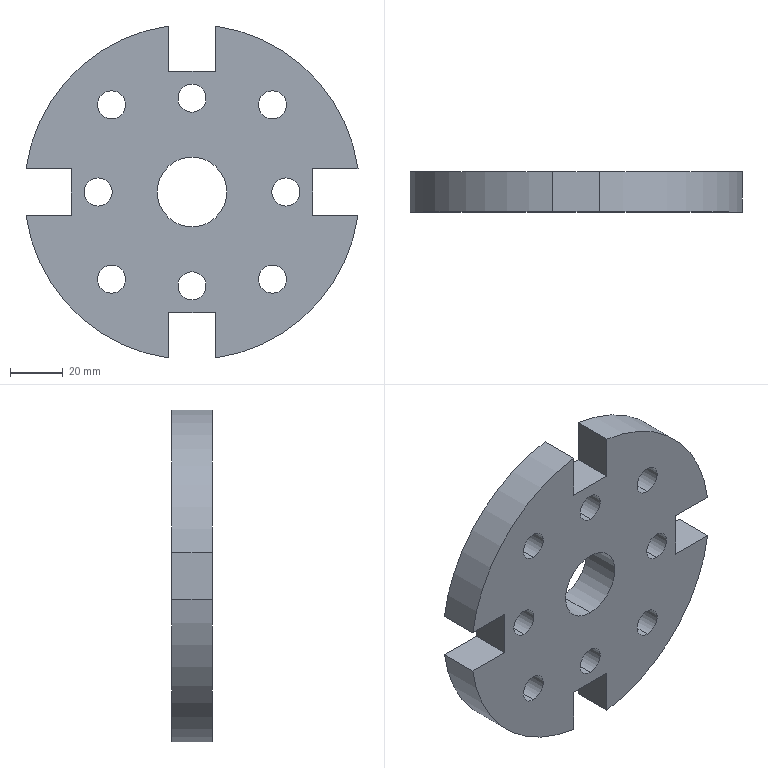Part | SolidWorks | features ICE 2, CirPattern 1, Extrusion 1, Scale 1 | 1 solid | 36 faces | box 125.749 x 15.24 x 125.749 mm | volume 154760 mm3 | cylinder 22 | plane 14 | commonest cylinder face diameters 10.668 x16 127 x4 26.416 x2
STEP:
#1=CARTESIAN_POINT('',(0.,-15.24,30.226));
#2=VERTEX_POINT('',#1);
#3=CARTESIAN_POINT('',(0.,-15.24,40.894));
#4=VERTEX_POINT('',#3);
#5=CARTESIAN_POINT('',(0.,-15.24,35.56));
#6=DIRECTION('',(0.,1.,0.));
#7=DIRECTION('',(0.,0.,1.));
#8=AXIS2_PLACEMENT_3D('',#5,#6,#7);
#9=CIRCLE('',#8,5.334);
#10=EDGE_CURVE('',#2,#4,#9,.T.);
#11=ORIENTED_EDGE('',*,*,#10,.F.);
#12=CARTESIAN_POINT('',(0.,0.,30.226));
#13=VERTEX_POINT('',#12);
#14=CARTESIAN_POINT('',(0.,-15.24,30.226));
#15=DIRECTION('',(0.,1.,0.));
#16=VECTOR('',#15,1000.);
#17=LINE('',#14,#16);
#18=EDGE_CURVE('',#2,#13,#17,.T.);
#19=ORIENTED_EDGE('',*,*,#18,.T.);
#20=CARTESIAN_POINT('',(0.,0.,40.894));
#21=VERTEX_POINT('',#20);
#22=CARTESIAN_POINT('',(0.,0.,35.56));
#23=DIRECTION('',(0.,1.,0.));
#24=DIRECTION('',(0.,0.,1.));
#25=AXIS2_PLACEMENT_3D('',#22,#23,#24);
#26=CIRCLE('',#25,5.334);
#27=EDGE_CURVE('',#13,#21,#26,.T.);
#28=ORIENTED_EDGE('',*,*,#27,.T.);
#29=CARTESIAN_POINT('',(0.,-15.24,40.894));
#30=DIRECTION('',(0.,1.,0.));
#31=VECTOR('',#30,1000.);
#32=LINE('',#29,#31);
#33=EDGE_CURVE('',#4,#21,#32,.T.);
#34=ORIENTED_EDGE('',*,*,#33,.F.);
#35=EDGE_LOOP('',(#11,#19,#28,#34));
#36=FACE_OUTER_BOUND('',#35,.T.);
#37=CARTESIAN_POINT('',(0.,-15.24,35.56));
#38=DIRECTION('',(0.,1.,0.));
#39=DIRECTION('',(0.,0.,1.));
#40=AXIS2_PLACEMENT_3D('',#37,#38,#39);
#41=CYLINDRICAL_SURFACE('',#40,5.334);
#42=ADVANCED_FACE('',(#36),#41,.F.);
#43=CARTESIAN_POINT('',(35.56,-15.24,-5.334));
#44=VERTEX_POINT('',#43);
#45=CARTESIAN_POINT('',(35.56,-15.24,5.334));
#46=VERTEX_POINT('',#45);
#47=CARTESIAN_POINT('',(35.56,-15.24,0.));
#48=DIRECTION('',(0.,1.,0.));
#49=DIRECTION('',(0.,0.,1.));
#50=AXIS2_PLACEMENT_3D('',#47,#48,#49);
#51=CIRCLE('',#50,5.334);
#52=EDGE_CURVE('',#44,#46,#51,.T.);
#53=ORIENTED_EDGE('',*,*,#52,.F.);
#54=CARTESIAN_POINT('',(35.56,0.,-5.334));
#55=VERTEX_POINT('',#54);
#56=CARTESIAN_POINT('',(35.56,-15.24,-5.334));
#57=DIRECTION('',(0.,1.,0.));
#58=VECTOR('',#57,1000.);
#59=LINE('',#56,#58);
#60=EDGE_CURVE('',#44,#55,#59,.T.);
#61=ORIENTED_EDGE('',*,*,#60,.T.);
#62=CARTESIAN_POINT('',(35.56,0.,5.334));
#63=VERTEX_POINT('',#62);
#64=CARTESIAN_POINT('',(35.56,0.,0.));
#65=DIRECTION('',(0.,1.,0.));
#66=DIRECTION('',(0.,0.,1.));
#67=AXIS2_PLACEMENT_3D('',#64,#65,#66);
#68=CIRCLE('',#67,5.334);
#69=EDGE_CURVE('',#55,#63,#68,.T.);
#70=ORIENTED_EDGE('',*,*,#69,.T.);
#71=CARTESIAN_POINT('',(35.56,-15.24,5.334));
#72=DIRECTION('',(0.,1.,0.));
#73=VECTOR('',#72,1000.);
#74=LINE('',#71,#73);
#75=EDGE_CURVE('',#46,#63,#74,.T.);
#76=ORIENTED_EDGE('',*,*,#75,.F.);
#77=EDGE_LOOP('',(#53,#61,#70,#76));
#78=FACE_OUTER_BOUND('',#77,.T.);
#79=CARTESIAN_POINT('',(35.56,-15.24,0.));
#80=DIRECTION('',(0.,1.,0.));
#81=DIRECTION('',(0.,0.,1.));
#82=AXIS2_PLACEMENT_3D('',#79,#80,#81);
#83=CYLINDRICAL_SURFACE('',#82,5.334);
#84=ADVANCED_FACE('',(#78),#83,.F.);
#85=CARTESIAN_POINT('',(0.,-15.24,-40.894));
#86=VERTEX_POINT('',#85);
#87=CARTESIAN_POINT('',(0.,-15.24,-30.226));
#88=VERTEX_POINT('',#87);
#89=CARTESIAN_POINT('',(0.,-15.24,-35.56));
#90=DIRECTION('',(0.,1.,0.));
#91=DIRECTION('',(0.,0.,1.));
#92=AXIS2_PLACEMENT_3D('',#89,#90,#91);
#93=CIRCLE('',#92,5.334);
#94=EDGE_CURVE('',#86,#88,#93,.T.);
#95=ORIENTED_EDGE('',*,*,#94,.F.);
#96=CARTESIAN_POINT('',(0.,0.,-40.894));
#97=VERTEX_POINT('',#96);
#98=CARTESIAN_POINT('',(0.,-15.24,-40.894));
#99=DIRECTION('',(0.,1.,0.));
#100=VECTOR('',#99,1000.);
#101=LINE('',#98,#100);
#102=EDGE_CURVE('',#86,#97,#101,.T.);
#103=ORIENTED_EDGE('',*,*,#102,.T.);
#104=CARTESIAN_POINT('',(0.,0.,-30.226));
#105=VERTEX_POINT('',#104);
#106=CARTESIAN_POINT('',(0.,0.,-35.56));
#107=DIRECTION('',(0.,1.,0.));
#108=DIRECTION('',(0.,0.,1.));
#109=AXIS2_PLACEMENT_3D('',#106,#107,#108);
#110=CIRCLE('',#109,5.334);
#111=EDGE_CURVE('',#97,#105,#110,.T.);
#112=ORIENTED_EDGE('',*,*,#111,.T.);
#113=CARTESIAN_POINT('',(0.,-15.24,-30.226));
#114=DIRECTION('',(0.,1.,0.));
#115=VECTOR('',#114,1000.);
#116=LINE('',#113,#115);
#117=EDGE_CURVE('',#88,#105,#116,.T.);
#118=ORIENTED_EDGE('',*,*,#117,.F.);
#119=EDGE_LOOP('',(#95,#103,#112,#118));
#120=FACE_OUTER_BOUND('',#119,.T.);
#121=CARTESIAN_POINT('',(0.,-15.24,-35.56));
#122=DIRECTION('',(0.,1.,0.));
#123=DIRECTION('',(0.,0.,1.));
#124=AXIS2_PLACEMENT_3D('',#121,#122,#123);
#125=CYLINDRICAL_SURFACE('',#124,5.334);
#126=ADVANCED_FACE('',(#120),#125,.F.);
#127=CARTESIAN_POINT('',(-35.56,-15.24,-5.334));
#128=VERTEX_POINT('',#127);
#129=CARTESIAN_POINT('',(-35.56,-15.24,5.334));
#130=VERTEX_POINT('',#129);
#131=CARTESIAN_POINT('',(-35.56,-15.24,0.));
#132=DIRECTION('',(0.,1.,0.));
#133=DIRECTION('',(0.,0.,1.));
#134=AXIS2_PLACEMENT_3D('',#131,#132,#133);
#135=CIRCLE('',#134,5.334);
#136=EDGE_CURVE('',#128,#130,#135,.T.);
#137=ORIENTED_EDGE('',*,*,#136,.F.);
#138=CARTESIAN_POINT('',(-35.56,0.,-5.334));
#139=VERTEX_POINT('',#138);
#140=CARTESIAN_POINT('',(-35.56,-15.24,-5.334));
#141=DIRECTION('',(0.,1.,0.));
#142=VECTOR('',#141,1000.);
#143=LINE('',#140,#142);
#144=EDGE_CURVE('',#128,#139,#143,.T.);
#145=ORIENTED_EDGE('',*,*,#144,.T.);
#146=CARTESIAN_POINT('',(-35.56,0.,5.334));
#147=VERTEX_POINT('',#146);
#148=CARTESIAN_POINT('',(-35.56,0.,0.));
#149=DIRECTION('',(0.,1.,0.));
#150=DIRECTION('',(0.,0.,1.));
#151=AXIS2_PLACEMENT_3D('',#148,#149,#150);
#152=CIRCLE('',#151,5.334);
#153=EDGE_CURVE('',#139,#147,#152,.T.);
#154=ORIENTED_EDGE('',*,*,#153,.T.);
#155=CARTESIAN_POINT('',(-35.56,-15.24,5.334));
#156=DIRECTION('',(0.,1.,0.));
#157=VECTOR('',#156,1000.);
#158=LINE('',#155,#157);
#159=EDGE_CURVE('',#130,#147,#158,.T.);
#160=ORIENTED_EDGE('',*,*,#159,.F.);
#161=EDGE_LOOP('',(#137,#145,#154,#160));
#162=FACE_OUTER_BOUND('',#161,.T.);
#163=CARTESIAN_POINT('',(-35.56,-15.24,0.));
#164=DIRECTION('',(0.,1.,0.));
#165=DIRECTION('',(0.,0.,1.));
#166=AXIS2_PLACEMENT_3D('',#163,#164,#165);
#167=CYLINDRICAL_SURFACE('',#166,5.334);
#168=ADVANCED_FACE('',(#162),#167,.F.);
#169=CARTESIAN_POINT('',(0.,-15.24,-13.208));
#170=VERTEX_POINT('',#169);
#171=CARTESIAN_POINT('',(0.,-15.24,13.208));
#172=VERTEX_POINT('',#171);
#173=CARTESIAN_POINT('',(0.,-15.24,0.));
#174=DIRECTION('',(0.,1.,0.));
#175=DIRECTION('',(0.,0.,1.));
#176=AXIS2_PLACEMENT_3D('',#173,#174,#175);
#177=CIRCLE('',#176,13.208);
#178=EDGE_CURVE('',#170,#172,#177,.T.);
#179=ORIENTED_EDGE('',*,*,#178,.F.);
#180=CARTESIAN_POINT('',(0.,0.,-13.208));
#181=VERTEX_POINT('',#180);
#182=CARTESIAN_POINT('',(0.,-15.24,-13.208));
#183=DIRECTION('',(0.,1.,0.));
#184=VECTOR('',#183,1000.);
#185=LINE('',#182,#184);
#186=EDGE_CURVE('',#170,#181,#185,.T.);
#187=ORIENTED_EDGE('',*,*,#186,.T.);
#188=CARTESIAN_POINT('',(0.,0.,13.208));
#189=VERTEX_POINT('',#188);
#190=CARTESIAN_POINT('',(0.,0.,0.));
#191=DIRECTION('',(0.,1.,0.));
#192=DIRECTION('',(0.,0.,1.));
#193=AXIS2_PLACEMENT_3D('',#190,#191,#192);
#194=CIRCLE('',#193,13.208);
#195=EDGE_CURVE('',#181,#189,#194,.T.);
#196=ORIENTED_EDGE('',*,*,#195,.T.);
#197=CARTESIAN_POINT('',(0.,-15.24,13.208));
#198=DIRECTION('',(0.,1.,0.));
#199=VECTOR('',#198,1000.);
#200=LINE('',#197,#199);
#201=EDGE_CURVE('',#172,#189,#200,.T.);
#202=ORIENTED_EDGE('',*,*,#201,.F.);
#203=EDGE_LOOP('',(#179,#187,#196,#202));
#204=FACE_OUTER_BOUND('',#203,.T.);
#205=CARTESIAN_POINT('',(0.,-15.24,0.));
#206=DIRECTION('',(0.,1.,0.));
#207=DIRECTION('',(0.,0.,1.));
#208=AXIS2_PLACEMENT_3D('',#205,#206,#207);
#209=CYLINDRICAL_SURFACE('',#208,13.208);
#210=ADVANCED_FACE('',(#204),#209,.F.);
#211=CARTESIAN_POINT('',(-30.48,-15.24,27.686));
#212=VERTEX_POINT('',#211);
#213=CARTESIAN_POINT('',(-30.48,-15.24,38.354));
#214=VERTEX_POINT('',#213);
#215=CARTESIAN_POINT('',(-30.48,-15.24,33.02));
#216=DIRECTION('',(0.,1.,0.));
#217=DIRECTION('',(0.,0.,1.));
#218=AXIS2_PLACEMENT_3D('',#215,#216,#217);
#219=CIRCLE('',#218,5.334);
#220=EDGE_CURVE('',#212,#214,#219,.T.);
#221=ORIENTED_EDGE('',*,*,#220,.F.);
#222=CARTESIAN_POINT('',(-30.48,0.,27.686));
#223=VERTEX_POINT('',#222);
#224=CARTESIAN_POINT('',(-30.48,-15.24,27.686));
#225=DIRECTION('',(0.,1.,0.));
#226=VECTOR('',#225,1000.);
#227=LINE('',#224,#226);
#228=EDGE_CURVE('',#212,#223,#227,.T.);
#229=ORIENTED_EDGE('',*,*,#228,.T.);
#230=CARTESIAN_POINT('',(-30.48,0.,38.354));
#231=VERTEX_POINT('',#230);
#232=CARTESIAN_POINT('',(-30.48,0.,33.02));
#233=DIRECTION('',(0.,1.,0.));
#234=DIRECTION('',(0.,0.,1.));
#235=AXIS2_PLACEMENT_3D('',#232,#233,#234);
#236=CIRCLE('',#235,5.334);
#237=EDGE_CURVE('',#223,#231,#236,.T.);
#238=ORIENTED_EDGE('',*,*,#237,.T.);
#239=CARTESIAN_POINT('',(-30.48,-15.24,38.354));
#240=DIRECTION('',(0.,1.,0.));
#241=VECTOR('',#240,1000.);
#242=LINE('',#239,#241);
#243=EDGE_CURVE('',#214,#231,#242,.T.);
#244=ORIENTED_EDGE('',*,*,#243,.F.);
#245=EDGE_LOOP('',(#221,#229,#238,#244));
#246=FACE_OUTER_BOUND('',#245,.T.);
#247=CARTESIAN_POINT('',(-30.48,-15.24,33.02));
#248=DIRECTION('',(0.,1.,0.));
#249=DIRECTION('',(0.,0.,1.));
#250=AXIS2_PLACEMENT_3D('',#247,#248,#249);
#251=CYLINDRICAL_SURFACE('',#250,5.334);
#252=ADVANCED_FACE('',(#246),#251,.F.);
#253=CARTESIAN_POINT('',(30.48,-15.24,27.686));
#254=VERTEX_POINT('',#253);
#255=CARTESIAN_POINT('',(30.48,-15.24,38.354));
#256=VERTEX_POINT('',#255);
#257=CARTESIAN_POINT('',(30.48,-15.24,33.02));
#258=DIRECTION('',(0.,1.,0.));
#259=DIRECTION('',(0.,0.,1.));
#260=AXIS2_PLACEMENT_3D('',#257,#258,#259);
#261=CIRCLE('',#260,5.334);
#262=EDGE_CURVE('',#254,#256,#261,.T.);
#263=ORIENTED_EDGE('',*,*,#262,.F.);
#264=CARTESIAN_POINT('',(30.48,0.,27.686));
#265=VERTEX_POINT('',#264);
#266=CARTESIAN_POINT('',(30.48,-15.24,27.686));
#267=DIRECTION('',(0.,1.,0.));
#268=VECTOR('',#267,1000.);
#269=LINE('',#266,#268);
#270=EDGE_CURVE('',#254,#265,#269,.T.);
#271=ORIENTED_EDGE('',*,*,#270,.T.);
#272=CARTESIAN_POINT('',(30.48,0.,38.354));
#273=VERTEX_POINT('',#272);
#274=CARTESIAN_POINT('',(30.48,0.,33.02));
#275=DIRECTION('',(0.,1.,0.));
#276=DIRECTION('',(0.,0.,1.));
#277=AXIS2_PLACEMENT_3D('',#274,#275,#276);
#278=CIRCLE('',#277,5.334);
#279=EDGE_CURVE('',#265,#273,#278,.T.);
#280=ORIENTED_EDGE('',*,*,#279,.T.);
#281=CARTESIAN_POINT('',(30.48,-15.24,38.354));
#282=DIRECTION('',(0.,1.,0.));
#283=VECTOR('',#282,1000.);
#284=LINE('',#281,#283);
#285=EDGE_CURVE('',#256,#273,#284,.T.);
#286=ORIENTED_EDGE('',*,*,#285,.F.);
#287=EDGE_LOOP('',(#263,#271,#280,#286));
#288=FACE_OUTER_BOUND('',#287,.T.);
#289=CARTESIAN_POINT('',(30.48,-15.24,33.02));
#290=DIRECTION('',(0.,1.,0.));
#291=DIRECTION('',(0.,0.,1.));
#292=AXIS2_PLACEMENT_3D('',#289,#290,#291);
#293=CYLINDRICAL_SURFACE('',#292,5.334);
#294=ADVANCED_FACE('',(#288),#293,.F.);
#295=CARTESIAN_POINT('',(30.48,-15.24,-38.354));
#296=VERTEX_POINT('',#295);
#297=CARTESIAN_POINT('',(30.48,-15.24,-27.686));
#298=VERTEX_POINT('',#297);
#299=CARTESIAN_POINT('',(30.48,-15.24,-33.02));
#300=DIRECTION('',(0.,1.,0.));
#301=DIRECTION('',(0.,0.,1.));
#302=AXIS2_PLACEMENT_3D('',#299,#300,#301);
#303=CIRCLE('',#302,5.334);
#304=EDGE_CURVE('',#296,#298,#303,.T.);
#305=ORIENTED_EDGE('',*,*,#304,.F.);
#306=CARTESIAN_POINT('',(30.48,0.,-38.354));
#307=VERTEX_POINT('',#306);
#308=CARTESIAN_POINT('',(30.48,-15.24,-38.354));
#309=DIRECTION('',(0.,1.,0.));
#310=VECTOR('',#309,1000.);
#311=LINE('',#308,#310);
#312=EDGE_CURVE('',#296,#307,#311,.T.);
#313=ORIENTED_EDGE('',*,*,#312,.T.);
#314=CARTESIAN_POINT('',(30.48,0.,-27.686));
#315=VERTEX_POINT('',#314);
#316=CARTESIAN_POINT('',(30.48,0.,-33.02));
#317=DIRECTION('',(0.,1.,0.));
#318=DIRECTION('',(0.,0.,1.));
#319=AXIS2_PLACEMENT_3D('',#316,#317,#318);
#320=CIRCLE('',#319,5.334);
#321=EDGE_CURVE('',#307,#315,#320,.T.);
#322=ORIENTED_EDGE('',*,*,#321,.T.);
#323=CARTESIAN_POINT('',(30.48,-15.24,-27.686));
#324=DIRECTION('',(0.,1.,0.));
#325=VECTOR('',#324,1000.);
#326=LINE('',#323,#325);
#327=EDGE_CURVE('',#298,#315,#326,.T.);
#328=ORIENTED_EDGE('',*,*,#327,.F.);
#329=EDGE_LOOP('',(#305,#313,#322,#328));
#330=FACE_OUTER_BOUND('',#329,.T.);
#331=CARTESIAN_POINT('',(30.48,-15.24,-33.02));
#332=DIRECTION('',(0.,1.,0.));
#333=DIRECTION('',(0.,0.,1.));
#334=AXIS2_PLACEMENT_3D('',#331,#332,#333);
#335=CYLINDRICAL_SURFACE('',#334,5.334);
#336=ADVANCED_FACE('',(#330),#335,.F.);
#337=CARTESIAN_POINT('',(-30.48,-15.24,-38.354));
#338=VERTEX_POINT('',#337);
#339=CARTESIAN_POINT('',(-30.48,-15.24,-27.686));
#340=VERTEX_POINT('',#339);
#341=CARTESIAN_POINT('',(-30.48,-15.24,-33.02));
#342=DIRECTION('',(0.,1.,0.));
#343=DIRECTION('',(0.,0.,1.));
#344=AXIS2_PLACEMENT_3D('',#341,#342,#343);
#345=CIRCLE('',#344,5.334);
#346=EDGE_CURVE('',#338,#340,#345,.T.);
#347=ORIENTED_EDGE('',*,*,#346,.F.);
#348=CARTESIAN_POINT('',(-30.48,0.,-38.354));
#349=VERTEX_POINT('',#348);
#350=CARTESIAN_POINT('',(-30.48,-15.24,-38.354));
#351=DIRECTION('',(0.,1.,0.));
#352=VECTOR('',#351,1000.);
#353=LINE('',#350,#352);
#354=EDGE_CURVE('',#338,#349,#353,.T.);
#355=ORIENTED_EDGE('',*,*,#354,.T.);
#356=CARTESIAN_POINT('',(-30.48,0.,-27.686));
#357=VERTEX_POINT('',#356);
#358=CARTESIAN_POINT('',(-30.48,0.,-33.02));
#359=DIRECTION('',(0.,1.,0.));
#360=DIRECTION('',(0.,0.,1.));
#361=AXIS2_PLACEMENT_3D('',#358,#359,#360);
#362=CIRCLE('',#361,5.334);
#363=EDGE_CURVE('',#349,#357,#362,.T.);
#364=ORIENTED_EDGE('',*,*,#363,.T.);
#365=CARTESIAN_POINT('',(-30.48,-15.24,-27.686));
#366=DIRECTION('',(0.,1.,0.));
#367=VECTOR('',#366,1000.);
#368=LINE('',#365,#367);
#369=EDGE_CURVE('',#340,#357,#368,.T.);
#370=ORIENTED_EDGE('',*,*,#369,.F.);
#371=EDGE_LOOP('',(#347,#355,#364,#370));
#372=FACE_OUTER_BOUND('',#371,.T.);
#373=CARTESIAN_POINT('',(-30.48,-15.24,-33.02));
#374=DIRECTION('',(0.,1.,0.));
#375=DIRECTION('',(0.,0.,1.));
#376=AXIS2_PLACEMENT_3D('',#373,#374,#375);
#377=CYLINDRICAL_SURFACE('',#376,5.334);
#378=ADVANCED_FACE('',(#372),#377,.F.);
#379=CARTESIAN_POINT('',(62.875,0.,8.89));
#380=VERTEX_POINT('',#379);
#381=CARTESIAN_POINT('',(62.875,-15.24,8.89));
#382=VERTEX_POINT('',#381);
#383=CARTESIAN_POINT('',(62.875,-15.24,8.89));
#384=DIRECTION('',(0.,-1.,0.));
#385=VECTOR('',#384,1000.);
#386=LINE('',#383,#385);
#387=EDGE_CURVE('',#380,#382,#386,.T.);
#388=ORIENTED_EDGE('',*,*,#387,.F.);
#389=CARTESIAN_POINT('',(8.89,0.,62.875));
#390=VERTEX_POINT('',#389);
#391=CARTESIAN_POINT('',(0.,0.,0.));
#392=DIRECTION('',(0.,1.,0.));
#393=DIRECTION('',(0.,0.,1.));
#394=AXIS2_PLACEMENT_3D('',#391,#392,#393);
#395=CIRCLE('',#394,63.5);
#396=EDGE_CURVE('',#390,#380,#395,.T.);
#397=ORIENTED_EDGE('',*,*,#396,.F.);
#398=CARTESIAN_POINT('',(8.89,-15.24,62.875));
#399=VERTEX_POINT('',#398);
#400=CARTESIAN_POINT('',(8.89,-15.24,62.875));
#401=DIRECTION('',(0.,1.,0.));
#402=VECTOR('',#401,1000.);
#403=LINE('',#400,#402);
#404=EDGE_CURVE('',#399,#390,#403,.T.);
#405=ORIENTED_EDGE('',*,*,#404,.F.);
#406=CARTESIAN_POINT('',(0.,-15.24,0.));
#407=DIRECTION('',(0.,1.,0.));
#408=DIRECTION('',(0.,0.,1.));
#409=AXIS2_PLACEMENT_3D('',#406,#407,#408);
#410=CIRCLE('',#409,63.5);
#411=EDGE_CURVE('',#399,#382,#410,.T.);
#412=ORIENTED_EDGE('',*,*,#411,.T.);
#413=EDGE_LOOP('',(#388,#397,#405,#412));
#414=FACE_OUTER_BOUND('',#413,.T.);
#415=CARTESIAN_POINT('',(0.,-15.24,0.));
#416=DIRECTION('',(0.,1.,0.));
#417=DIRECTION('',(0.,0.,1.));
#418=AXIS2_PLACEMENT_3D('',#415,#416,#417);
#419=CYLINDRICAL_SURFACE('',#418,63.5);
#420=ADVANCED_FACE('',(#414),#419,.T.);
#421=CARTESIAN_POINT('',(-8.89,0.,62.875));
#422=VERTEX_POINT('',#421);
#423=CARTESIAN_POINT('',(-8.89,-15.24,62.875));
#424=VERTEX_POINT('',#423);
#425=CARTESIAN_POINT('',(-8.89,-15.24,62.875));
#426=DIRECTION('',(0.,-1.,0.));
#427=VECTOR('',#426,1000.);
#428=LINE('',#425,#427);
#429=EDGE_CURVE('',#422,#424,#428,.T.);
#430=ORIENTED_EDGE('',*,*,#429,.F.);
#431=CARTESIAN_POINT('',(-62.875,0.,8.89));
#432=VERTEX_POINT('',#431);
#433=CARTESIAN_POINT('',(0.,0.,0.));
#434=DIRECTION('',(0.,1.,0.));
#435=DIRECTION('',(0.,0.,1.));
#436=AXIS2_PLACEMENT_3D('',#433,#434,#435);
#437=CIRCLE('',#436,63.5);
#438=EDGE_CURVE('',#432,#422,#437,.T.);
#439=ORIENTED_EDGE('',*,*,#438,.F.);
#440=CARTESIAN_POINT('',(-62.875,-15.24,8.89));
#441=VERTEX_POINT('',#440);
#442=CARTESIAN_POINT('',(-62.875,-15.24,8.89));
#443=DIRECTION('',(0.,1.,0.));
#444=VECTOR('',#443,1000.);
#445=LINE('',#442,#444);
#446=EDGE_CURVE('',#441,#432,#445,.T.);
#447=ORIENTED_EDGE('',*,*,#446,.F.);
#448=CARTESIAN_POINT('',(0.,-15.24,0.));
#449=DIRECTION('',(0.,1.,0.));
#450=DIRECTION('',(0.,0.,1.));
#451=AXIS2_PLACEMENT_3D('',#448,#449,#450);
#452=CIRCLE('',#451,63.5);
#453=EDGE_CURVE('',#441,#424,#452,.T.);
#454=ORIENTED_EDGE('',*,*,#453,.T.);
#455=EDGE_LOOP('',(#430,#439,#447,#454));
#456=FACE_OUTER_BOUND('',#455,.T.);
#457=CARTESIAN_POINT('',(0.,-15.24,0.));
#458=DIRECTION('',(0.,1.,0.));
#459=DIRECTION('',(0.,0.,1.));
#460=AXIS2_PLACEMENT_3D('',#457,#458,#459);
#461=CYLINDRICAL_SURFACE('',#460,63.5);
#462=ADVANCED_FACE('',(#456),#461,.T.);
#463=CARTESIAN_POINT('',(-62.875,0.,-8.89));
#464=VERTEX_POINT('',#463);
#465=CARTESIAN_POINT('',(-62.875,-15.24,-8.89));
#466=VERTEX_POINT('',#465);
#467=CARTESIAN_POINT('',(-62.875,-15.24,-8.89));
#468=DIRECTION('',(0.,-1.,0.));
#469=VECTOR('',#468,1000.);
#470=LINE('',#467,#469);
#471=EDGE_CURVE('',#464,#466,#470,.T.);
#472=ORIENTED_EDGE('',*,*,#471,.F.);
#473=CARTESIAN_POINT('',(-8.89,0.,-62.875));
#474=VERTEX_POINT('',#473);
#475=CARTESIAN_POINT('',(0.,0.,0.));
#476=DIRECTION('',(0.,1.,0.));
#477=DIRECTION('',(0.,0.,1.));
#478=AXIS2_PLACEMENT_3D('',#475,#476,#477);
#479=CIRCLE('',#478,63.5);
#480=EDGE_CURVE('',#474,#464,#479,.T.);
#481=ORIENTED_EDGE('',*,*,#480,.F.);
#482=CARTESIAN_POINT('',(-8.89,-15.24,-62.875));
#483=VERTEX_POINT('',#482);
#484=CARTESIAN_POINT('',(-8.89,-15.24,-62.875));
#485=DIRECTION('',(0.,1.,0.));
#486=VECTOR('',#485,1000.);
#487=LINE('',#484,#486);
#488=EDGE_CURVE('',#483,#474,#487,.T.);
#489=ORIENTED_EDGE('',*,*,#488,.F.);
#490=CARTESIAN_POINT('',(0.,-15.24,0.));
#491=DIRECTION('',(0.,1.,0.));
#492=DIRECTION('',(0.,0.,1.));
#493=AXIS2_PLACEMENT_3D('',#490,#491,#492);
#494=CIRCLE('',#493,63.5);
#495=EDGE_CURVE('',#483,#466,#494,.T.);
#496=ORIENTED_EDGE('',*,*,#495,.T.);
#497=EDGE_LOOP('',(#472,#481,#489,#496));
#498=FACE_OUTER_BOUND('',#497,.T.);
#499=CARTESIAN_POINT('',(0.,-15.24,0.));
#500=DIRECTION('',(0.,1.,0.));
#501=DIRECTION('',(0.,0.,1.));
#502=AXIS2_PLACEMENT_3D('',#499,#500,#501);
#503=CYLINDRICAL_SURFACE('',#502,63.5);
#504=ADVANCED_FACE('',(#498),#503,.T.);
#505=CARTESIAN_POINT('',(62.875,-15.24,-8.89));
#506=VERTEX_POINT('',#505);
#507=CARTESIAN_POINT('',(62.875,0.,-8.89));
#508=VERTEX_POINT('',#507);
#509=CARTESIAN_POINT('',(62.875,-15.24,-8.89));
#510=DIRECTION('',(0.,1.,0.));
#511=VECTOR('',#510,1000.);
#512=LINE('',#509,#511);
#513=EDGE_CURVE('',#506,#508,#512,.T.);
#514=ORIENTED_EDGE('',*,*,#513,.F.);
#515=CARTESIAN_POINT('',(8.89,-15.24,-62.875));
#516=VERTEX_POINT('',#515);
#517=CARTESIAN_POINT('',(0.,-15.24,0.));
#518=DIRECTION('',(0.,1.,0.));
#519=DIRECTION('',(0.,0.,1.));
#520=AXIS2_PLACEMENT_3D('',#517,#518,#519);
#521=CIRCLE('',#520,63.5);
#522=EDGE_CURVE('',#506,#516,#521,.T.);
#523=ORIENTED_EDGE('',*,*,#522,.T.);
#524=CARTESIAN_POINT('',(8.89,0.,-62.875));
#525=VERTEX_POINT('',#524);
#526=CARTESIAN_POINT('',(8.89,-15.24,-62.875));
#527=DIRECTION('',(0.,-1.,0.));
#528=VECTOR('',#527,1000.);
#529=LINE('',#526,#528);
#530=EDGE_CURVE('',#525,#516,#529,.T.);
#531=ORIENTED_EDGE('',*,*,#530,.F.);
#532=CARTESIAN_POINT('',(0.,0.,0.));
#533=DIRECTION('',(0.,1.,0.));
#534=DIRECTION('',(0.,0.,1.));
#535=AXIS2_PLACEMENT_3D('',#532,#533,#534);
#536=CIRCLE('',#535,63.5);
#537=EDGE_CURVE('',#508,#525,#536,.T.);
#538=ORIENTED_EDGE('',*,*,#537,.F.);
#539=EDGE_LOOP('',(#514,#523,#531,#538));
#540=FACE_OUTER_BOUND('',#539,.T.);
#541=CARTESIAN_POINT('',(0.,-15.24,0.));
#542=DIRECTION('',(0.,1.,0.));
#543=DIRECTION('',(0.,0.,1.));
#544=AXIS2_PLACEMENT_3D('',#541,#542,#543);
#545=CYLINDRICAL_SURFACE('',#544,63.5);
#546=ADVANCED_FACE('',(#540),#545,.T.);
#547=CARTESIAN_POINT('',(0.,-15.24,35.56));
#548=DIRECTION('',(0.,1.,0.));
#549=DIRECTION('',(0.,0.,1.));
#550=AXIS2_PLACEMENT_3D('',#547,#548,#549);
#551=CIRCLE('',#550,5.334);
#552=EDGE_CURVE('',#4,#2,#551,.T.);
#553=ORIENTED_EDGE('',*,*,#552,.T.);
#554=ORIENTED_EDGE('',*,*,#10,.T.);
#555=EDGE_LOOP('',(#553,#554));
#556=FACE_BOUND('',#555,.T.);
#557=CARTESIAN_POINT('',(35.56,-15.24,0.));
#558=DIRECTION('',(0.,1.,0.));
#559=DIRECTION('',(0.,0.,1.));
#560=AXIS2_PLACEMENT_3D('',#557,#558,#559);
#561=CIRCLE('',#560,5.334);
#562=EDGE_CURVE('',#46,#44,#561,.T.);
#563=ORIENTED_EDGE('',*,*,#562,.T.);
#564=ORIENTED_EDGE('',*,*,#52,.T.);
#565=EDGE_LOOP('',(#563,#564));
#566=FACE_BOUND('',#565,.T.);
#567=CARTESIAN_POINT('',(0.,-15.24,-35.56));
#568=DIRECTION('',(0.,1.,0.));
#569=DIRECTION('',(0.,0.,1.));
#570=AXIS2_PLACEMENT_3D('',#567,#568,#569);
#571=CIRCLE('',#570,5.334);
#572=EDGE_CURVE('',#88,#86,#571,.T.);
#573=ORIENTED_EDGE('',*,*,#572,.T.);
#574=ORIENTED_EDGE('',*,*,#94,.T.);
#575=EDGE_LOOP('',(#573,#574));
#576=FACE_BOUND('',#575,.T.);
#577=CARTESIAN_POINT('',(-35.56,-15.24,0.));
#578=DIRECTION('',(0.,1.,0.));
#579=DIRECTION('',(0.,0.,1.));
#580=AXIS2_PLACEMENT_3D('',#577,#578,#579);
#581=CIRCLE('',#580,5.334);
#582=EDGE_CURVE('',#130,#128,#581,.T.);
#583=ORIENTED_EDGE('',*,*,#582,.T.);
#584=ORIENTED_EDGE('',*,*,#136,.T.);
#585=EDGE_LOOP('',(#583,#584));
#586=FACE_BOUND('',#585,.T.);
#587=CARTESIAN_POINT('',(0.,-15.24,0.));
#588=DIRECTION('',(0.,1.,0.));
#589=DIRECTION('',(0.,0.,1.));
#590=AXIS2_PLACEMENT_3D('',#587,#588,#589);
#591=CIRCLE('',#590,13.208);
#592=EDGE_CURVE('',#172,#170,#591,.T.);
#593=ORIENTED_EDGE('',*,*,#592,.T.);
#594=ORIENTED_EDGE('',*,*,#178,.T.);
#595=EDGE_LOOP('',(#593,#594));
#596=FACE_BOUND('',#595,.T.);
#597=CARTESIAN_POINT('',(-30.48,-15.24,33.02));
#598=DIRECTION('',(0.,1.,0.));
#599=DIRECTION('',(0.,0.,1.));
#600=AXIS2_PLACEMENT_3D('',#597,#598,#599);
#601=CIRCLE('',#600,5.334);
#602=EDGE_CURVE('',#214,#212,#601,.T.);
#603=ORIENTED_EDGE('',*,*,#602,.T.);
#604=ORIENTED_EDGE('',*,*,#220,.T.);
#605=EDGE_LOOP('',(#603,#604));
#606=FACE_BOUND('',#605,.T.);
#607=CARTESIAN_POINT('',(30.48,-15.24,33.02));
#608=DIRECTION('',(0.,1.,0.));
#609=DIRECTION('',(0.,0.,1.));
#610=AXIS2_PLACEMENT_3D('',#607,#608,#609);
#611=CIRCLE('',#610,5.334);
#612=EDGE_CURVE('',#256,#254,#611,.T.);
#613=ORIENTED_EDGE('',*,*,#612,.T.);
#614=ORIENTED_EDGE('',*,*,#262,.T.);
#615=EDGE_LOOP('',(#613,#614));
#616=FACE_BOUND('',#615,.T.);
#617=CARTESIAN_POINT('',(30.48,-15.24,-33.02));
#618=DIRECTION('',(0.,1.,0.));
#619=DIRECTION('',(0.,0.,1.));
#620=AXIS2_PLACEMENT_3D('',#617,#618,#619);
#621=CIRCLE('',#620,5.334);
#622=EDGE_CURVE('',#298,#296,#621,.T.);
#623=ORIENTED_EDGE('',*,*,#622,.T.);
#624=ORIENTED_EDGE('',*,*,#304,.T.);
#625=EDGE_LOOP('',(#623,#624));
#626=FACE_BOUND('',#625,.T.);
#627=CARTESIAN_POINT('',(-30.48,-15.24,-33.02));
#628=DIRECTION('',(0.,1.,0.));
#629=DIRECTION('',(0.,0.,1.));
#630=AXIS2_PLACEMENT_3D('',#627,#628,#629);
#631=CIRCLE('',#630,5.334);
#632=EDGE_CURVE('',#340,#338,#631,.T.);
#633=ORIENTED_EDGE('',*,*,#632,.T.);
#634=ORIENTED_EDGE('',*,*,#346,.T.);
#635=EDGE_LOOP('',(#633,#634));
#636=FACE_BOUND('',#635,.T.);
#637=CARTESIAN_POINT('',(45.72,-15.24,-8.89));
#638=VERTEX_POINT('',#637);
#639=CARTESIAN_POINT('',(45.72,-15.24,8.89));
#640=VERTEX_POINT('',#639);
#641=CARTESIAN_POINT('',(45.72,-15.24,-8.89));
#642=DIRECTION('',(0.,0.,1.));
#643=VECTOR('',#642,1000.);
#644=LINE('',#641,#643);
#645=EDGE_CURVE('',#638,#640,#644,.T.);
#646=ORIENTED_EDGE('',*,*,#645,.T.);
#647=CARTESIAN_POINT('',(81.28,-15.24,8.89));
#648=DIRECTION('',(1.,0.,0.));
#649=VECTOR('',#648,1000.);
#650=LINE('',#647,#649);
#651=EDGE_CURVE('',#640,#382,#650,.T.);
#652=ORIENTED_EDGE('',*,*,#651,.T.);
#653=ORIENTED_EDGE('',*,*,#411,.F.);
#654=CARTESIAN_POINT('',(8.89,-15.24,45.72));
#655=VERTEX_POINT('',#654);
#656=CARTESIAN_POINT('',(8.89,-15.24,81.28));
#657=DIRECTION('',(0.,0.,-1.));
#658=VECTOR('',#657,1000.);
#659=LINE('',#656,#658);
#660=EDGE_CURVE('',#399,#655,#659,.T.);
#661=ORIENTED_EDGE('',*,*,#660,.T.);
#662=CARTESIAN_POINT('',(-8.89,-15.24,45.72));
#663=VERTEX_POINT('',#662);
#664=CARTESIAN_POINT('',(8.89,-15.24,45.72));
#665=DIRECTION('',(-1.,0.,0.));
#666=VECTOR('',#665,1000.);
#667=LINE('',#664,#666);
#668=EDGE_CURVE('',#655,#663,#667,.T.);
#669=ORIENTED_EDGE('',*,*,#668,.T.);
#670=CARTESIAN_POINT('',(-8.89,-15.24,81.28));
#671=DIRECTION('',(0.,0.,1.));
#672=VECTOR('',#671,1000.);
#673=LINE('',#670,#672);
#674=EDGE_CURVE('',#663,#424,#673,.T.);
#675=ORIENTED_EDGE('',*,*,#674,.T.);
#676=ORIENTED_EDGE('',*,*,#453,.F.);
#677=CARTESIAN_POINT('',(-45.72,-15.24,8.89));
#678=VERTEX_POINT('',#677);
#679=CARTESIAN_POINT('',(-81.28,-15.24,8.89));
#680=DIRECTION('',(1.,0.,0.));
#681=VECTOR('',#680,1000.);
#682=LINE('',#679,#681);
#683=EDGE_CURVE('',#441,#678,#682,.T.);
#684=ORIENTED_EDGE('',*,*,#683,.T.);
#685=CARTESIAN_POINT('',(-45.72,-15.24,-8.89));
#686=VERTEX_POINT('',#685);
#687=CARTESIAN_POINT('',(-45.72,-15.24,8.89));
#688=DIRECTION('',(0.,0.,-1.));
#689=VECTOR('',#688,1000.);
#690=LINE('',#687,#689);
#691=EDGE_CURVE('',#678,#686,#690,.T.);
#692=ORIENTED_EDGE('',*,*,#691,.T.);
#693=CARTESIAN_POINT('',(-81.28,-15.24,-8.89));
#694=DIRECTION('',(-1.,0.,0.));
#695=VECTOR('',#694,1000.);
#696=LINE('',#693,#695);
#697=EDGE_CURVE('',#686,#466,#696,.T.);
#698=ORIENTED_EDGE('',*,*,#697,.T.);
#699=ORIENTED_EDGE('',*,*,#495,.F.);
#700=CARTESIAN_POINT('',(-8.89,-15.24,-45.72));
#701=VERTEX_POINT('',#700);
#702=CARTESIAN_POINT('',(-8.89,-15.24,-81.28));
#703=DIRECTION('',(0.,0.,1.));
#704=VECTOR('',#703,1000.);
#705=LINE('',#702,#704);
#706=EDGE_CURVE('',#483,#701,#705,.T.);
#707=ORIENTED_EDGE('',*,*,#706,.T.);
#708=CARTESIAN_POINT('',(8.89,-15.24,-45.72));
#709=VERTEX_POINT('',#708);
#710=CARTESIAN_POINT('',(-8.89,-15.24,-45.72));
#711=DIRECTION('',(1.,0.,0.));
#712=VECTOR('',#711,1000.);
#713=LINE('',#710,#712);
#714=EDGE_CURVE('',#701,#709,#713,.T.);
#715=ORIENTED_EDGE('',*,*,#714,.T.);
#716=CARTESIAN_POINT('',(8.89,-15.24,-81.28));
#717=DIRECTION('',(0.,0.,-1.));
#718=VECTOR('',#717,1000.);
#719=LINE('',#716,#718);
#720=EDGE_CURVE('',#709,#516,#719,.T.);
#721=ORIENTED_EDGE('',*,*,#720,.T.);
#722=ORIENTED_EDGE('',*,*,#522,.F.);
#723=CARTESIAN_POINT('',(81.28,-15.24,-8.89));
#724=DIRECTION('',(-1.,0.,0.));
#725=VECTOR('',#724,1000.);
#726=LINE('',#723,#725);
#727=EDGE_CURVE('',#506,#638,#726,.T.);
#728=ORIENTED_EDGE('',*,*,#727,.T.);
#729=EDGE_LOOP('',(#646,#652,#653,#661,#669,#675,#676,#684,#692,#698,#699,#707,#715,#721,#722,#728));
#730=FACE_OUTER_BOUND('',#729,.T.);
#731=CARTESIAN_POINT('',(0.,-15.24,0.));
#732=DIRECTION('',(0.,1.,0.));
#733=DIRECTION('',(0.,0.,1.));
#734=AXIS2_PLACEMENT_3D('',#731,#732,#733);
#735=PLANE('',#734);
#736=ADVANCED_FACE('',(#556,#566,#576,#586,#596,#606,#616,#626,#636,#730),#735,.F.);
#737=CARTESIAN_POINT('',(45.72,0.,8.89));
#738=VERTEX_POINT('',#737);
#739=CARTESIAN_POINT('',(81.28,0.,8.89));
#740=DIRECTION('',(1.,0.,0.));
#741=VECTOR('',#740,1000.);
#742=LINE('',#739,#741);
#743=EDGE_CURVE('',#738,#380,#742,.T.);
#744=ORIENTED_EDGE('',*,*,#743,.F.);
#745=CARTESIAN_POINT('',(45.72,0.,-8.89));
#746=VERTEX_POINT('',#745);
#747=CARTESIAN_POINT('',(45.72,0.,-8.89));
#748=DIRECTION('',(0.,0.,1.));
#749=VECTOR('',#748,1000.);
#750=LINE('',#747,#749);
#751=EDGE_CURVE('',#746,#738,#750,.T.);
#752=ORIENTED_EDGE('',*,*,#751,.F.);
#753=CARTESIAN_POINT('',(0.,0.,-8.89));
#754=DIRECTION('',(-1.,0.,0.));
#755=VECTOR('',#754,1000.);
#756=LINE('',#753,#755);
#757=EDGE_CURVE('',#508,#746,#756,.T.);
#758=ORIENTED_EDGE('',*,*,#757,.F.);
#759=ORIENTED_EDGE('',*,*,#537,.T.);
#760=CARTESIAN_POINT('',(8.89,0.,-45.72));
#761=VERTEX_POINT('',#760);
#762=CARTESIAN_POINT('',(8.89,0.,-81.28));
#763=DIRECTION('',(0.,0.,-1.));
#764=VECTOR('',#763,1000.);
#765=LINE('',#762,#764);
#766=EDGE_CURVE('',#761,#525,#765,.T.);
#767=ORIENTED_EDGE('',*,*,#766,.F.);
#768=CARTESIAN_POINT('',(-8.89,0.,-45.72));
#769=VERTEX_POINT('',#768);
#770=CARTESIAN_POINT('',(-8.89,0.,-45.72));
#771=DIRECTION('',(1.,0.,0.));
#772=VECTOR('',#771,1000.);
#773=LINE('',#770,#772);
#774=EDGE_CURVE('',#769,#761,#773,.T.);
#775=ORIENTED_EDGE('',*,*,#774,.F.);
#776=CARTESIAN_POINT('',(-8.89,0.,0.));
#777=DIRECTION('',(0.,0.,1.));
#778=VECTOR('',#777,1000.);
#779=LINE('',#776,#778);
#780=EDGE_CURVE('',#474,#769,#779,.T.);
#781=ORIENTED_EDGE('',*,*,#780,.F.);
#782=ORIENTED_EDGE('',*,*,#480,.T.);
#783=CARTESIAN_POINT('',(-45.72,0.,-8.89));
#784=VERTEX_POINT('',#783);
#785=CARTESIAN_POINT('',(-81.28,0.,-8.89));
#786=DIRECTION('',(-1.,0.,0.));
#787=VECTOR('',#786,1000.);
#788=LINE('',#785,#787);
#789=EDGE_CURVE('',#784,#464,#788,.T.);
#790=ORIENTED_EDGE('',*,*,#789,.F.);
#791=CARTESIAN_POINT('',(-45.72,0.,8.89));
#792=VERTEX_POINT('',#791);
#793=CARTESIAN_POINT('',(-45.72,0.,8.89));
#794=DIRECTION('',(0.,0.,-1.));
#795=VECTOR('',#794,1000.);
#796=LINE('',#793,#795);
#797=EDGE_CURVE('',#792,#784,#796,.T.);
#798=ORIENTED_EDGE('',*,*,#797,.F.);
#799=CARTESIAN_POINT('',(0.,0.,8.89));
#800=DIRECTION('',(1.,0.,0.));
#801=VECTOR('',#800,1000.);
#802=LINE('',#799,#801);
#803=EDGE_CURVE('',#432,#792,#802,.T.);
#804=ORIENTED_EDGE('',*,*,#803,.F.);
#805=ORIENTED_EDGE('',*,*,#438,.T.);
#806=CARTESIAN_POINT('',(-8.89,0.,45.72));
#807=VERTEX_POINT('',#806);
#808=CARTESIAN_POINT('',(-8.89,0.,81.28));
#809=DIRECTION('',(0.,0.,1.));
#810=VECTOR('',#809,1000.);
#811=LINE('',#808,#810);
#812=EDGE_CURVE('',#807,#422,#811,.T.);
#813=ORIENTED_EDGE('',*,*,#812,.F.);
#814=CARTESIAN_POINT('',(8.89,0.,45.72));
#815=VERTEX_POINT('',#814);
#816=CARTESIAN_POINT('',(8.89,0.,45.72));
#817=DIRECTION('',(-1.,0.,0.));
#818=VECTOR('',#817,1000.);
#819=LINE('',#816,#818);
#820=EDGE_CURVE('',#815,#807,#819,.T.);
#821=ORIENTED_EDGE('',*,*,#820,.F.);
#822=CARTESIAN_POINT('',(8.89,0.,0.));
#823=DIRECTION('',(0.,0.,-1.));
#824=VECTOR('',#823,1000.);
#825=LINE('',#822,#824);
#826=EDGE_CURVE('',#390,#815,#825,.T.);
#827=ORIENTED_EDGE('',*,*,#826,.F.);
#828=ORIENTED_EDGE('',*,*,#396,.T.);
#829=EDGE_LOOP('',(#744,#752,#758,#759,#767,#775,#781,#782,#790,#798,#804,#805,#813,#821,#827,#828));
#830=FACE_OUTER_BOUND('',#829,.T.);
#831=CARTESIAN_POINT('',(0.,0.,35.56));
#832=DIRECTION('',(0.,1.,0.));
#833=DIRECTION('',(0.,0.,1.));
#834=AXIS2_PLACEMENT_3D('',#831,#832,#833);
#835=CIRCLE('',#834,5.334);
#836=EDGE_CURVE('',#21,#13,#835,.T.);
#837=ORIENTED_EDGE('',*,*,#836,.F.);
#838=ORIENTED_EDGE('',*,*,#27,.F.);
#839=EDGE_LOOP('',(#837,#838));
#840=FACE_BOUND('',#839,.T.);
#841=CARTESIAN_POINT('',(35.56,0.,0.));
#842=DIRECTION('',(0.,1.,0.));
#843=DIRECTION('',(0.,0.,1.));
#844=AXIS2_PLACEMENT_3D('',#841,#842,#843);
#845=CIRCLE('',#844,5.334);
#846=EDGE_CURVE('',#63,#55,#845,.T.);
#847=ORIENTED_EDGE('',*,*,#846,.F.);
#848=ORIENTED_EDGE('',*,*,#69,.F.);
#849=EDGE_LOOP('',(#847,#848));
#850=FACE_BOUND('',#849,.T.);
#851=CARTESIAN_POINT('',(0.,0.,-35.56));
#852=DIRECTION('',(0.,1.,0.));
#853=DIRECTION('',(0.,0.,1.));
#854=AXIS2_PLACEMENT_3D('',#851,#852,#853);
#855=CIRCLE('',#854,5.334);
#856=EDGE_CURVE('',#105,#97,#855,.T.);
#857=ORIENTED_EDGE('',*,*,#856,.F.);
#858=ORIENTED_EDGE('',*,*,#111,.F.);
#859=EDGE_LOOP('',(#857,#858));
#860=FACE_BOUND('',#859,.T.);
#861=CARTESIAN_POINT('',(-35.56,0.,0.));
#862=DIRECTION('',(0.,1.,0.));
#863=DIRECTION('',(0.,0.,1.));
#864=AXIS2_PLACEMENT_3D('',#861,#862,#863);
#865=CIRCLE('',#864,5.334);
#866=EDGE_CURVE('',#147,#139,#865,.T.);
#867=ORIENTED_EDGE('',*,*,#866,.F.);
#868=ORIENTED_EDGE('',*,*,#153,.F.);
#869=EDGE_LOOP('',(#867,#868));
#870=FACE_BOUND('',#869,.T.);
#871=CARTESIAN_POINT('',(0.,0.,0.));
#872=DIRECTION('',(0.,1.,0.));
#873=DIRECTION('',(0.,0.,1.));
#874=AXIS2_PLACEMENT_3D('',#871,#872,#873);
#875=CIRCLE('',#874,13.208);
#876=EDGE_CURVE('',#189,#181,#875,.T.);
#877=ORIENTED_EDGE('',*,*,#876,.F.);
#878=ORIENTED_EDGE('',*,*,#195,.F.);
#879=EDGE_LOOP('',(#877,#878));
#880=FACE_BOUND('',#879,.T.);
#881=CARTESIAN_POINT('',(-30.48,0.,33.02));
#882=DIRECTION('',(0.,1.,0.));
#883=DIRECTION('',(0.,0.,1.));
#884=AXIS2_PLACEMENT_3D('',#881,#882,#883);
#885=CIRCLE('',#884,5.334);
#886=EDGE_CURVE('',#231,#223,#885,.T.);
#887=ORIENTED_EDGE('',*,*,#886,.F.);
#888=ORIENTED_EDGE('',*,*,#237,.F.);
#889=EDGE_LOOP('',(#887,#888));
#890=FACE_BOUND('',#889,.T.);
#891=CARTESIAN_POINT('',(30.48,0.,33.02));
#892=DIRECTION('',(0.,1.,0.));
#893=DIRECTION('',(0.,0.,1.));
#894=AXIS2_PLACEMENT_3D('',#891,#892,#893);
#895=CIRCLE('',#894,5.334);
#896=EDGE_CURVE('',#273,#265,#895,.T.);
#897=ORIENTED_EDGE('',*,*,#896,.F.);
#898=ORIENTED_EDGE('',*,*,#279,.F.);
#899=EDGE_LOOP('',(#897,#898));
#900=FACE_BOUND('',#899,.T.);
#901=CARTESIAN_POINT('',(30.48,0.,-33.02));
#902=DIRECTION('',(0.,1.,0.));
#903=DIRECTION('',(0.,0.,1.));
#904=AXIS2_PLACEMENT_3D('',#901,#902,#903);
#905=CIRCLE('',#904,5.334);
#906=EDGE_CURVE('',#315,#307,#905,.T.);
#907=ORIENTED_EDGE('',*,*,#906,.F.);
#908=ORIENTED_EDGE('',*,*,#321,.F.);
#909=EDGE_LOOP('',(#907,#908));
#910=FACE_BOUND('',#909,.T.);
#911=CARTESIAN_POINT('',(-30.48,0.,-33.02));
#912=DIRECTION('',(0.,1.,0.));
#913=DIRECTION('',(0.,0.,1.));
#914=AXIS2_PLACEMENT_3D('',#911,#912,#913);
#915=CIRCLE('',#914,5.334);
#916=EDGE_CURVE('',#357,#349,#915,.T.);
#917=ORIENTED_EDGE('',*,*,#916,.F.);
#918=ORIENTED_EDGE('',*,*,#363,.F.);
#919=EDGE_LOOP('',(#917,#918));
#920=FACE_BOUND('',#919,.T.);
#921=CARTESIAN_POINT('',(0.,0.,0.));
#922=DIRECTION('',(0.,1.,0.));
#923=DIRECTION('',(0.,0.,1.));
#924=AXIS2_PLACEMENT_3D('',#921,#922,#923);
#925=PLANE('',#924);
#926=ADVANCED_FACE('',(#830,#840,#850,#860,#870,#880,#890,#900,#910,#920),#925,.T.);
#927=ORIENTED_EDGE('',*,*,#354,.F.);
#928=ORIENTED_EDGE('',*,*,#632,.F.);
#929=ORIENTED_EDGE('',*,*,#369,.T.);
#930=ORIENTED_EDGE('',*,*,#916,.T.);
#931=EDGE_LOOP('',(#927,#928,#929,#930));
#932=FACE_OUTER_BOUND('',#931,.T.);
#933=CARTESIAN_POINT('',(-30.48,-15.24,-33.02));
#934=DIRECTION('',(0.,1.,0.));
#935=DIRECTION('',(0.,0.,1.));
#936=AXIS2_PLACEMENT_3D('',#933,#934,#935);
#937=CYLINDRICAL_SURFACE('',#936,5.334);
#938=ADVANCED_FACE('',(#932),#937,.F.);
#939=ORIENTED_EDGE('',*,*,#312,.F.);
#940=ORIENTED_EDGE('',*,*,#622,.F.);
#941=ORIENTED_EDGE('',*,*,#327,.T.);
#942=ORIENTED_EDGE('',*,*,#906,.T.);
#943=EDGE_LOOP('',(#939,#940,#941,#942));
#944=FACE_OUTER_BOUND('',#943,.T.);
#945=CARTESIAN_POINT('',(30.48,-15.24,-33.02));
#946=DIRECTION('',(0.,1.,0.));
#947=DIRECTION('',(0.,0.,1.));
#948=AXIS2_PLACEMENT_3D('',#945,#946,#947);
#949=CYLINDRICAL_SURFACE('',#948,5.334);
#950=ADVANCED_FACE('',(#944),#949,.F.);
#951=ORIENTED_EDGE('',*,*,#270,.F.);
#952=ORIENTED_EDGE('',*,*,#612,.F.);
#953=ORIENTED_EDGE('',*,*,#285,.T.);
#954=ORIENTED_EDGE('',*,*,#896,.T.);
#955=EDGE_LOOP('',(#951,#952,#953,#954));
#956=FACE_OUTER_BOUND('',#955,.T.);
#957=CARTESIAN_POINT('',(30.48,-15.24,33.02));
#958=DIRECTION('',(0.,1.,0.));
#959=DIRECTION('',(0.,0.,1.));
#960=AXIS2_PLACEMENT_3D('',#957,#958,#959);
#961=CYLINDRICAL_SURFACE('',#960,5.334);
#962=ADVANCED_FACE('',(#956),#961,.F.);
#963=ORIENTED_EDGE('',*,*,#228,.F.);
#964=ORIENTED_EDGE('',*,*,#602,.F.);
#965=ORIENTED_EDGE('',*,*,#243,.T.);
#966=ORIENTED_EDGE('',*,*,#886,.T.);
#967=EDGE_LOOP('',(#963,#964,#965,#966));
#968=FACE_OUTER_BOUND('',#967,.T.);
#969=CARTESIAN_POINT('',(-30.48,-15.24,33.02));
#970=DIRECTION('',(0.,1.,0.));
#971=DIRECTION('',(0.,0.,1.));
#972=AXIS2_PLACEMENT_3D('',#969,#970,#971);
#973=CYLINDRICAL_SURFACE('',#972,5.334);
#974=ADVANCED_FACE('',(#968),#973,.F.);
#975=ORIENTED_EDGE('',*,*,#530,.T.);
#976=ORIENTED_EDGE('',*,*,#720,.F.);
#977=CARTESIAN_POINT('',(8.89,-15.24,-45.72));
#978=DIRECTION('',(0.,1.,0.));
#979=VECTOR('',#978,1000.);
#980=LINE('',#977,#979);
#981=EDGE_CURVE('',#709,#761,#980,.T.);
#982=ORIENTED_EDGE('',*,*,#981,.T.);
#983=ORIENTED_EDGE('',*,*,#766,.T.);
#984=EDGE_LOOP('',(#975,#976,#982,#983));
#985=FACE_OUTER_BOUND('',#984,.T.);
#986=CARTESIAN_POINT('',(8.89,-15.24,-81.28));
#987=DIRECTION('',(1.,0.,0.));
#988=DIRECTION('',(0.,0.,-1.));
#989=AXIS2_PLACEMENT_3D('',#986,#987,#988);
#990=PLANE('',#989);
#991=ADVANCED_FACE('',(#985),#990,.F.);
#992=ORIENTED_EDGE('',*,*,#774,.T.);
#993=ORIENTED_EDGE('',*,*,#981,.F.);
#994=ORIENTED_EDGE('',*,*,#714,.F.);
#995=CARTESIAN_POINT('',(-8.89,-15.24,-45.72));
#996=DIRECTION('',(0.,1.,0.));
#997=VECTOR('',#996,1000.);
#998=LINE('',#995,#997);
#999=EDGE_CURVE('',#701,#769,#998,.T.);
#1000=ORIENTED_EDGE('',*,*,#999,.T.);
#1001=EDGE_LOOP('',(#992,#993,#994,#1000));
#1002=FACE_OUTER_BOUND('',#1001,.T.);
#1003=CARTESIAN_POINT('',(-8.89,-15.24,-45.72));
#1004=DIRECTION('',(0.,0.,1.));
#1005=DIRECTION('',(1.,0.,0.));
#1006=AXIS2_PLACEMENT_3D('',#1003,#1004,#1005);
#1007=PLANE('',#1006);
#1008=ADVANCED_FACE('',(#1002),#1007,.F.);
#1009=ORIENTED_EDGE('',*,*,#488,.T.);
#1010=ORIENTED_EDGE('',*,*,#780,.T.);
#1011=ORIENTED_EDGE('',*,*,#999,.F.);
#1012=ORIENTED_EDGE('',*,*,#706,.F.);
#1013=EDGE_LOOP('',(#1009,#1010,#1011,#1012));
#1014=FACE_OUTER_BOUND('',#1013,.T.);
#1015=CARTESIAN_POINT('',(-8.89,-15.24,-81.28));
#1016=DIRECTION('',(-1.,0.,0.));
#1017=DIRECTION('',(0.,0.,1.));
#1018=AXIS2_PLACEMENT_3D('',#1015,#1016,#1017);
#1019=PLANE('',#1018);
#1020=ADVANCED_FACE('',(#1014),#1019,.F.);
#1021=ORIENTED_EDGE('',*,*,#186,.F.);
#1022=ORIENTED_EDGE('',*,*,#592,.F.);
#1023=ORIENTED_EDGE('',*,*,#201,.T.);
#1024=ORIENTED_EDGE('',*,*,#876,.T.);
#1025=EDGE_LOOP('',(#1021,#1022,#1023,#1024));
#1026=FACE_OUTER_BOUND('',#1025,.T.);
#1027=CARTESIAN_POINT('',(0.,-15.24,0.));
#1028=DIRECTION('',(0.,1.,0.));
#1029=DIRECTION('',(0.,0.,1.));
#1030=AXIS2_PLACEMENT_3D('',#1027,#1028,#1029);
#1031=CYLINDRICAL_SURFACE('',#1030,13.208);
#1032=ADVANCED_FACE('',(#1026),#1031,.F.);
#1033=ORIENTED_EDGE('',*,*,#144,.F.);
#1034=ORIENTED_EDGE('',*,*,#582,.F.);
#1035=ORIENTED_EDGE('',*,*,#159,.T.);
#1036=ORIENTED_EDGE('',*,*,#866,.T.);
#1037=EDGE_LOOP('',(#1033,#1034,#1035,#1036));
#1038=FACE_OUTER_BOUND('',#1037,.T.);
#1039=CARTESIAN_POINT('',(-35.56,-15.24,0.));
#1040=DIRECTION('',(0.,1.,0.));
#1041=DIRECTION('',(0.,0.,1.));
#1042=AXIS2_PLACEMENT_3D('',#1039,#1040,#1041);
#1043=CYLINDRICAL_SURFACE('',#1042,5.334);
#1044=ADVANCED_FACE('',(#1038),#1043,.F.);
#1045=ORIENTED_EDGE('',*,*,#102,.F.);
#1046=ORIENTED_EDGE('',*,*,#572,.F.);
#1047=ORIENTED_EDGE('',*,*,#117,.T.);
#1048=ORIENTED_EDGE('',*,*,#856,.T.);
#1049=EDGE_LOOP('',(#1045,#1046,#1047,#1048));
#1050=FACE_OUTER_BOUND('',#1049,.T.);
#1051=CARTESIAN_POINT('',(0.,-15.24,-35.56));
#1052=DIRECTION('',(0.,1.,0.));
#1053=DIRECTION('',(0.,0.,1.));
#1054=AXIS2_PLACEMENT_3D('',#1051,#1052,#1053);
#1055=CYLINDRICAL_SURFACE('',#1054,5.334);
#1056=ADVANCED_FACE('',(#1050),#1055,.F.);
#1057=ORIENTED_EDGE('',*,*,#60,.F.);
#1058=ORIENTED_EDGE('',*,*,#562,.F.);
#1059=ORIENTED_EDGE('',*,*,#75,.T.);
#1060=ORIENTED_EDGE('',*,*,#846,.T.);
#1061=EDGE_LOOP('',(#1057,#1058,#1059,#1060));
#1062=FACE_OUTER_BOUND('',#1061,.T.);
#1063=CARTESIAN_POINT('',(35.56,-15.24,0.));
#1064=DIRECTION('',(0.,1.,0.));
#1065=DIRECTION('',(0.,0.,1.));
#1066=AXIS2_PLACEMENT_3D('',#1063,#1064,#1065);
#1067=CYLINDRICAL_SURFACE('',#1066,5.334);
#1068=ADVANCED_FACE('',(#1062),#1067,.F.);
#1069=ORIENTED_EDGE('',*,*,#18,.F.);
#1070=ORIENTED_EDGE('',*,*,#552,.F.);
#1071=ORIENTED_EDGE('',*,*,#33,.T.);
#1072=ORIENTED_EDGE('',*,*,#836,.T.);
#1073=EDGE_LOOP('',(#1069,#1070,#1071,#1072));
#1074=FACE_OUTER_BOUND('',#1073,.T.);
#1075=CARTESIAN_POINT('',(0.,-15.24,35.56));
#1076=DIRECTION('',(0.,1.,0.));
#1077=DIRECTION('',(0.,0.,1.));
#1078=AXIS2_PLACEMENT_3D('',#1075,#1076,#1077);
#1079=CYLINDRICAL_SURFACE('',#1078,5.334);
#1080=ADVANCED_FACE('',(#1074),#1079,.F.);
#1081=ORIENTED_EDGE('',*,*,#471,.T.);
#1082=ORIENTED_EDGE('',*,*,#697,.F.);
#1083=CARTESIAN_POINT('',(-45.72,-15.24,-8.89));
#1084=DIRECTION('',(0.,1.,0.));
#1085=VECTOR('',#1084,1000.);
#1086=LINE('',#1083,#1085);
#1087=EDGE_CURVE('',#686,#784,#1086,.T.);
#1088=ORIENTED_EDGE('',*,*,#1087,.T.);
#1089=ORIENTED_EDGE('',*,*,#789,.T.);
#1090=EDGE_LOOP('',(#1081,#1082,#1088,#1089));
#1091=FACE_OUTER_BOUND('',#1090,.T.);
#1092=CARTESIAN_POINT('',(-81.28,-15.24,-8.89));
#1093=DIRECTION('',(0.,0.,-1.));
#1094=DIRECTION('',(-1.,0.,0.));
#1095=AXIS2_PLACEMENT_3D('',#1092,#1093,#1094);
#1096=PLANE('',#1095);
#1097=ADVANCED_FACE('',(#1091),#1096,.F.);
#1098=ORIENTED_EDGE('',*,*,#797,.T.);
#1099=ORIENTED_EDGE('',*,*,#1087,.F.);
#1100=ORIENTED_EDGE('',*,*,#691,.F.);
#1101=CARTESIAN_POINT('',(-45.72,-15.24,8.89));
#1102=DIRECTION('',(0.,1.,0.));
#1103=VECTOR('',#1102,1000.);
#1104=LINE('',#1101,#1103);
#1105=EDGE_CURVE('',#678,#792,#1104,.T.);
#1106=ORIENTED_EDGE('',*,*,#1105,.T.);
#1107=EDGE_LOOP('',(#1098,#1099,#1100,#1106));
#1108=FACE_OUTER_BOUND('',#1107,.T.);
#1109=CARTESIAN_POINT('',(-45.72,-15.24,8.89));
#1110=DIRECTION('',(1.,0.,0.));
#1111=DIRECTION('',(0.,0.,-1.));
#1112=AXIS2_PLACEMENT_3D('',#1109,#1110,#1111);
#1113=PLANE('',#1112);
#1114=ADVANCED_FACE('',(#1108),#1113,.F.);
#1115=ORIENTED_EDGE('',*,*,#446,.T.);
#1116=ORIENTED_EDGE('',*,*,#803,.T.);
#1117=ORIENTED_EDGE('',*,*,#1105,.F.);
#1118=ORIENTED_EDGE('',*,*,#683,.F.);
#1119=EDGE_LOOP('',(#1115,#1116,#1117,#1118));
#1120=FACE_OUTER_BOUND('',#1119,.T.);
#1121=CARTESIAN_POINT('',(-81.28,-15.24,8.89));
#1122=DIRECTION('',(0.,0.,1.));
#1123=DIRECTION('',(1.,0.,0.));
#1124=AXIS2_PLACEMENT_3D('',#1121,#1122,#1123);
#1125=PLANE('',#1124);
#1126=ADVANCED_FACE('',(#1120),#1125,.F.);
#1127=ORIENTED_EDGE('',*,*,#429,.T.);
#1128=ORIENTED_EDGE('',*,*,#674,.F.);
#1129=CARTESIAN_POINT('',(-8.89,-15.24,45.72));
#1130=DIRECTION('',(0.,1.,0.));
#1131=VECTOR('',#1130,1000.);
#1132=LINE('',#1129,#1131);
#1133=EDGE_CURVE('',#663,#807,#1132,.T.);
#1134=ORIENTED_EDGE('',*,*,#1133,.T.);
#1135=ORIENTED_EDGE('',*,*,#812,.T.);
#1136=EDGE_LOOP('',(#1127,#1128,#1134,#1135));
#1137=FACE_OUTER_BOUND('',#1136,.T.);
#1138=CARTESIAN_POINT('',(-8.89,-15.24,81.28));
#1139=DIRECTION('',(-1.,0.,0.));
#1140=DIRECTION('',(0.,0.,1.));
#1141=AXIS2_PLACEMENT_3D('',#1138,#1139,#1140);
#1142=PLANE('',#1141);
#1143=ADVANCED_FACE('',(#1137),#1142,.F.);
#1144=ORIENTED_EDGE('',*,*,#820,.T.);
#1145=ORIENTED_EDGE('',*,*,#1133,.F.);
#1146=ORIENTED_EDGE('',*,*,#668,.F.);
#1147=CARTESIAN_POINT('',(8.89,-15.24,45.72));
#1148=DIRECTION('',(0.,1.,0.));
#1149=VECTOR('',#1148,1000.);
#1150=LINE('',#1147,#1149);
#1151=EDGE_CURVE('',#655,#815,#1150,.T.);
#1152=ORIENTED_EDGE('',*,*,#1151,.T.);
#1153=EDGE_LOOP('',(#1144,#1145,#1146,#1152));
#1154=FACE_OUTER_BOUND('',#1153,.T.);
#1155=CARTESIAN_POINT('',(8.89,-15.24,45.72));
#1156=DIRECTION('',(0.,0.,-1.));
#1157=DIRECTION('',(-1.,0.,0.));
#1158=AXIS2_PLACEMENT_3D('',#1155,#1156,#1157);
#1159=PLANE('',#1158);
#1160=ADVANCED_FACE('',(#1154),#1159,.F.);
#1161=ORIENTED_EDGE('',*,*,#404,.T.);
#1162=ORIENTED_EDGE('',*,*,#826,.T.);
#1163=ORIENTED_EDGE('',*,*,#1151,.F.);
#1164=ORIENTED_EDGE('',*,*,#660,.F.);
#1165=EDGE_LOOP('',(#1161,#1162,#1163,#1164));
#1166=FACE_OUTER_BOUND('',#1165,.T.);
#1167=CARTESIAN_POINT('',(8.89,-15.24,81.28));
#1168=DIRECTION('',(1.,0.,0.));
#1169=DIRECTION('',(0.,0.,-1.));
#1170=AXIS2_PLACEMENT_3D('',#1167,#1168,#1169);
#1171=PLANE('',#1170);
#1172=ADVANCED_FACE('',(#1166),#1171,.F.);
#1173=ORIENTED_EDGE('',*,*,#387,.T.);
#1174=ORIENTED_EDGE('',*,*,#651,.F.);
#1175=CARTESIAN_POINT('',(45.72,-15.24,8.89));
#1176=DIRECTION('',(0.,1.,0.));
#1177=VECTOR('',#1176,1000.);
#1178=LINE('',#1175,#1177);
#1179=EDGE_CURVE('',#640,#738,#1178,.T.);
#1180=ORIENTED_EDGE('',*,*,#1179,.T.);
#1181=ORIENTED_EDGE('',*,*,#743,.T.);
#1182=EDGE_LOOP('',(#1173,#1174,#1180,#1181));
#1183=FACE_OUTER_BOUND('',#1182,.T.);
#1184=CARTESIAN_POINT('',(81.28,-15.24,8.89));
#1185=DIRECTION('',(0.,0.,1.));
#1186=DIRECTION('',(1.,0.,0.));
#1187=AXIS2_PLACEMENT_3D('',#1184,#1185,#1186);
#1188=PLANE('',#1187);
#1189=ADVANCED_FACE('',(#1183),#1188,.F.);
#1190=ORIENTED_EDGE('',*,*,#751,.T.);
#1191=ORIENTED_EDGE('',*,*,#1179,.F.);
#1192=ORIENTED_EDGE('',*,*,#645,.F.);
#1193=CARTESIAN_POINT('',(45.72,-15.24,-8.89));
#1194=DIRECTION('',(0.,1.,0.));
#1195=VECTOR('',#1194,1000.);
#1196=LINE('',#1193,#1195);
#1197=EDGE_CURVE('',#638,#746,#1196,.T.);
#1198=ORIENTED_EDGE('',*,*,#1197,.T.);
#1199=EDGE_LOOP('',(#1190,#1191,#1192,#1198));
#1200=FACE_OUTER_BOUND('',#1199,.T.);
#1201=CARTESIAN_POINT('',(45.72,-15.24,-8.89));
#1202=DIRECTION('',(-1.,0.,0.));
#1203=DIRECTION('',(0.,0.,1.));
#1204=AXIS2_PLACEMENT_3D('',#1201,#1202,#1203);
#1205=PLANE('',#1204);
#1206=ADVANCED_FACE('',(#1200),#1205,.F.);
#1207=ORIENTED_EDGE('',*,*,#513,.T.);
#1208=ORIENTED_EDGE('',*,*,#757,.T.);
#1209=ORIENTED_EDGE('',*,*,#1197,.F.);
#1210=ORIENTED_EDGE('',*,*,#727,.F.);
#1211=EDGE_LOOP('',(#1207,#1208,#1209,#1210));
#1212=FACE_OUTER_BOUND('',#1211,.T.);
#1213=CARTESIAN_POINT('',(81.28,-15.24,-8.89));
#1214=DIRECTION('',(0.,0.,-1.));
#1215=DIRECTION('',(-1.,0.,0.));
#1216=AXIS2_PLACEMENT_3D('',#1213,#1214,#1215);
#1217=PLANE('',#1216);
#1218=ADVANCED_FACE('',(#1212),#1217,.F.);
#1219=CLOSED_SHELL('',(#42,#84,#126,#168,#210,#252,#294,#336,#378,#420,#462,#504,#546,#736,#926,#938,#950,#962,#974,#991,#1008,#1020,#1032,#1044,#1056,#1068,#1080,#1097,#1114,#1126,#1143,#1160,#1172,#1189,#1206,#1218));
#1220=MANIFOLD_SOLID_BREP('',#1219);
#1221=CARTESIAN_POINT('',(0.,0.,0.));
#1222=DIRECTION('',(0.,0.,1.));
#1223=DIRECTION('',(1.,0.,0.));
#1224=AXIS2_PLACEMENT_3D('',#1221,#1222,#1223);
#1225=(LENGTH_UNIT()NAMED_UNIT(*)SI_UNIT(.MILLI.,.METRE.));
#1226=UNCERTAINTY_MEASURE_WITH_UNIT(LENGTH_MEASURE(0.00001),#1225,'','');
#1227=(NAMED_UNIT(*)PLANE_ANGLE_UNIT()SI_UNIT($,.RADIAN.));
#1228=(NAMED_UNIT(*)SI_UNIT($,.STERADIAN.)SOLID_ANGLE_UNIT());
#1229=(GEOMETRIC_REPRESENTATION_CONTEXT(3)GLOBAL_UNCERTAINTY_ASSIGNED_CONTEXT((#1226))GLOBAL_UNIT_ASSIGNED_CONTEXT((#1225,#1227,#1228))REPRESENTATION_CONTEXT('',''));
#1230=ADVANCED_BREP_SHAPE_REPRESENTATION('',(#1220,#1224),#1229);